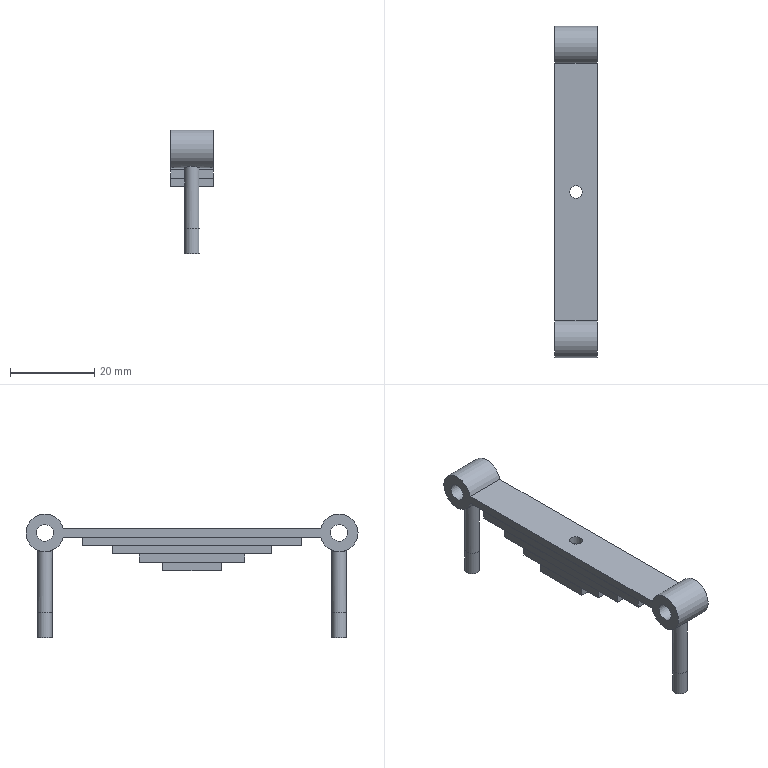Part | STEP file | 1-41.1 | 5 solids | 43 faces | box 10 x 79 x 29.5 mm | volume 5148 mm3 | plane 30 | cylinder 13 | commonest cylinder face diameters 3 x5 3.5 x4 4 x2 9 x2